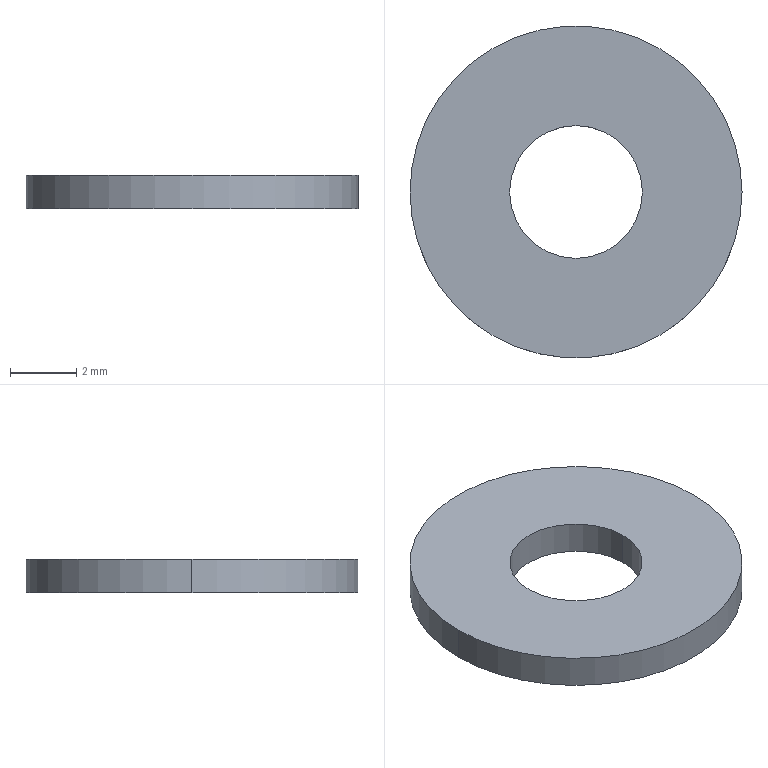Part | SolidWorks | features BaseBody 1 | 1 solid | 6 faces | box 10 x 10 x 1 mm | volume 65.973 mm3 | cylinder 4 | plane 2 | commonest cylinder face diameters 4 x2 10 x2
STEP:
#1=CARTESIAN_POINT('',(2.,0.,1.));
#2=VERTEX_POINT('',#1);
#3=CARTESIAN_POINT('',(2.,0.,0.));
#4=VERTEX_POINT('',#3);
#5=CARTESIAN_POINT('',(2.,0.,1.));
#6=DIRECTION('',(0.,0.,-1.));
#7=VECTOR('',#6,1000.);
#8=LINE('',#5,#7);
#9=EDGE_CURVE('',#2,#4,#8,.T.);
#10=ORIENTED_EDGE('',*,*,#9,.F.);
#11=CARTESIAN_POINT('',(-2.,0.,1.));
#12=VERTEX_POINT('',#11);
#13=CARTESIAN_POINT('',(0.,0.,1.));
#14=DIRECTION('',(0.,0.,1.));
#15=DIRECTION('',(1.,0.,0.));
#16=AXIS2_PLACEMENT_3D('',#13,#14,#15);
#17=CIRCLE('',#16,2.);
#18=EDGE_CURVE('',#2,#12,#17,.T.);
#19=ORIENTED_EDGE('',*,*,#18,.T.);
#20=CARTESIAN_POINT('',(-2.,0.,0.));
#21=VERTEX_POINT('',#20);
#22=CARTESIAN_POINT('',(-2.,0.,1.));
#23=DIRECTION('',(0.,0.,-1.));
#24=VECTOR('',#23,1000.);
#25=LINE('',#22,#24);
#26=EDGE_CURVE('',#12,#21,#25,.T.);
#27=ORIENTED_EDGE('',*,*,#26,.T.);
#28=CARTESIAN_POINT('',(0.,0.,0.));
#29=DIRECTION('',(0.,0.,1.));
#30=DIRECTION('',(1.,0.,0.));
#31=AXIS2_PLACEMENT_3D('',#28,#29,#30);
#32=CIRCLE('',#31,2.);
#33=EDGE_CURVE('',#4,#21,#32,.T.);
#34=ORIENTED_EDGE('',*,*,#33,.F.);
#35=EDGE_LOOP('',(#10,#19,#27,#34));
#36=FACE_OUTER_BOUND('',#35,.T.);
#37=CARTESIAN_POINT('',(0.,0.,1.));
#38=DIRECTION('',(0.,0.,-1.));
#39=DIRECTION('',(-1.,0.,0.));
#40=AXIS2_PLACEMENT_3D('',#37,#38,#39);
#41=CYLINDRICAL_SURFACE('',#40,2.);
#42=ADVANCED_FACE('',(#36),#41,.F.);
#43=CARTESIAN_POINT('',(5.,0.,1.));
#44=VERTEX_POINT('',#43);
#45=CARTESIAN_POINT('',(5.,0.,0.));
#46=VERTEX_POINT('',#45);
#47=CARTESIAN_POINT('',(5.,0.,1.));
#48=DIRECTION('',(0.,0.,-1.));
#49=VECTOR('',#48,1000.);
#50=LINE('',#47,#49);
#51=EDGE_CURVE('',#44,#46,#50,.T.);
#52=ORIENTED_EDGE('',*,*,#51,.F.);
#53=CARTESIAN_POINT('',(-5.,0.,1.));
#54=VERTEX_POINT('',#53);
#55=CARTESIAN_POINT('',(0.,0.,1.));
#56=DIRECTION('',(0.,0.,1.));
#57=DIRECTION('',(1.,0.,0.));
#58=AXIS2_PLACEMENT_3D('',#55,#56,#57);
#59=CIRCLE('',#58,5.);
#60=EDGE_CURVE('',#54,#44,#59,.T.);
#61=ORIENTED_EDGE('',*,*,#60,.F.);
#62=CARTESIAN_POINT('',(-5.,0.,0.));
#63=VERTEX_POINT('',#62);
#64=CARTESIAN_POINT('',(-5.,0.,1.));
#65=DIRECTION('',(0.,0.,-1.));
#66=VECTOR('',#65,1000.);
#67=LINE('',#64,#66);
#68=EDGE_CURVE('',#54,#63,#67,.T.);
#69=ORIENTED_EDGE('',*,*,#68,.T.);
#70=CARTESIAN_POINT('',(0.,0.,0.));
#71=DIRECTION('',(0.,0.,1.));
#72=DIRECTION('',(1.,0.,0.));
#73=AXIS2_PLACEMENT_3D('',#70,#71,#72);
#74=CIRCLE('',#73,5.);
#75=EDGE_CURVE('',#63,#46,#74,.T.);
#76=ORIENTED_EDGE('',*,*,#75,.T.);
#77=EDGE_LOOP('',(#52,#61,#69,#76));
#78=FACE_OUTER_BOUND('',#77,.T.);
#79=CARTESIAN_POINT('',(0.,0.,1.));
#80=DIRECTION('',(0.,0.,-1.));
#81=DIRECTION('',(-1.,0.,0.));
#82=AXIS2_PLACEMENT_3D('',#79,#80,#81);
#83=CYLINDRICAL_SURFACE('',#82,5.);
#84=ADVANCED_FACE('',(#78),#83,.T.);
#85=CARTESIAN_POINT('',(0.,0.,0.));
#86=DIRECTION('',(0.,0.,1.));
#87=DIRECTION('',(1.,0.,0.));
#88=AXIS2_PLACEMENT_3D('',#85,#86,#87);
#89=CIRCLE('',#88,2.);
#90=EDGE_CURVE('',#21,#4,#89,.T.);
#91=ORIENTED_EDGE('',*,*,#90,.T.);
#92=ORIENTED_EDGE('',*,*,#33,.T.);
#93=EDGE_LOOP('',(#91,#92));
#94=FACE_BOUND('',#93,.T.);
#95=ORIENTED_EDGE('',*,*,#75,.F.);
#96=CARTESIAN_POINT('',(0.,0.,0.));
#97=DIRECTION('',(0.,0.,1.));
#98=DIRECTION('',(1.,0.,0.));
#99=AXIS2_PLACEMENT_3D('',#96,#97,#98);
#100=CIRCLE('',#99,5.);
#101=EDGE_CURVE('',#46,#63,#100,.T.);
#102=ORIENTED_EDGE('',*,*,#101,.F.);
#103=EDGE_LOOP('',(#95,#102));
#104=FACE_OUTER_BOUND('',#103,.T.);
#105=CARTESIAN_POINT('',(0.,0.,0.));
#106=DIRECTION('',(0.,0.,1.));
#107=DIRECTION('',(1.,0.,0.));
#108=AXIS2_PLACEMENT_3D('',#105,#106,#107);
#109=PLANE('',#108);
#110=ADVANCED_FACE('',(#94,#104),#109,.F.);
#111=CARTESIAN_POINT('',(0.,0.,1.));
#112=DIRECTION('',(0.,0.,1.));
#113=DIRECTION('',(1.,0.,0.));
#114=AXIS2_PLACEMENT_3D('',#111,#112,#113);
#115=CIRCLE('',#114,2.);
#116=EDGE_CURVE('',#12,#2,#115,.T.);
#117=ORIENTED_EDGE('',*,*,#116,.F.);
#118=ORIENTED_EDGE('',*,*,#18,.F.);
#119=EDGE_LOOP('',(#117,#118));
#120=FACE_BOUND('',#119,.T.);
#121=ORIENTED_EDGE('',*,*,#60,.T.);
#122=CARTESIAN_POINT('',(0.,0.,1.));
#123=DIRECTION('',(0.,0.,1.));
#124=DIRECTION('',(1.,0.,0.));
#125=AXIS2_PLACEMENT_3D('',#122,#123,#124);
#126=CIRCLE('',#125,5.);
#127=EDGE_CURVE('',#44,#54,#126,.T.);
#128=ORIENTED_EDGE('',*,*,#127,.T.);
#129=EDGE_LOOP('',(#121,#128));
#130=FACE_OUTER_BOUND('',#129,.T.);
#131=CARTESIAN_POINT('',(0.,0.,1.));
#132=DIRECTION('',(0.,0.,1.));
#133=DIRECTION('',(1.,0.,0.));
#134=AXIS2_PLACEMENT_3D('',#131,#132,#133);
#135=PLANE('',#134);
#136=ADVANCED_FACE('',(#120,#130),#135,.T.);
#137=ORIENTED_EDGE('',*,*,#127,.F.);
#138=ORIENTED_EDGE('',*,*,#51,.T.);
#139=ORIENTED_EDGE('',*,*,#101,.T.);
#140=ORIENTED_EDGE('',*,*,#68,.F.);
#141=EDGE_LOOP('',(#137,#138,#139,#140));
#142=FACE_OUTER_BOUND('',#141,.T.);
#143=CARTESIAN_POINT('',(0.,0.,1.));
#144=DIRECTION('',(0.,0.,-1.));
#145=DIRECTION('',(-1.,0.,0.));
#146=AXIS2_PLACEMENT_3D('',#143,#144,#145);
#147=CYLINDRICAL_SURFACE('',#146,5.);
#148=ADVANCED_FACE('',(#142),#147,.T.);
#149=ORIENTED_EDGE('',*,*,#116,.T.);
#150=ORIENTED_EDGE('',*,*,#9,.T.);
#151=ORIENTED_EDGE('',*,*,#90,.F.);
#152=ORIENTED_EDGE('',*,*,#26,.F.);
#153=EDGE_LOOP('',(#149,#150,#151,#152));
#154=FACE_OUTER_BOUND('',#153,.T.);
#155=CARTESIAN_POINT('',(0.,0.,1.));
#156=DIRECTION('',(0.,0.,-1.));
#157=DIRECTION('',(-1.,0.,0.));
#158=AXIS2_PLACEMENT_3D('',#155,#156,#157);
#159=CYLINDRICAL_SURFACE('',#158,2.);
#160=ADVANCED_FACE('',(#154),#159,.F.);
#161=CLOSED_SHELL('',(#42,#84,#110,#136,#148,#160));
#162=MANIFOLD_SOLID_BREP('',#161);
#163=CARTESIAN_POINT('',(0.,0.,0.));
#164=DIRECTION('',(0.,0.,1.));
#165=DIRECTION('',(1.,0.,0.));
#166=AXIS2_PLACEMENT_3D('',#163,#164,#165);
#167=(LENGTH_UNIT()NAMED_UNIT(*)SI_UNIT(.MILLI.,.METRE.));
#168=UNCERTAINTY_MEASURE_WITH_UNIT(LENGTH_MEASURE(0.00001),#167,'','');
#169=(NAMED_UNIT(*)PLANE_ANGLE_UNIT()SI_UNIT($,.RADIAN.));
#170=(NAMED_UNIT(*)SI_UNIT($,.STERADIAN.)SOLID_ANGLE_UNIT());
#171=(GEOMETRIC_REPRESENTATION_CONTEXT(3)GLOBAL_UNCERTAINTY_ASSIGNED_CONTEXT((#168))GLOBAL_UNIT_ASSIGNED_CONTEXT((#167,#169,#170))REPRESENTATION_CONTEXT('',''));
#172=ADVANCED_BREP_SHAPE_REPRESENTATION('',(#162,#166),#171);